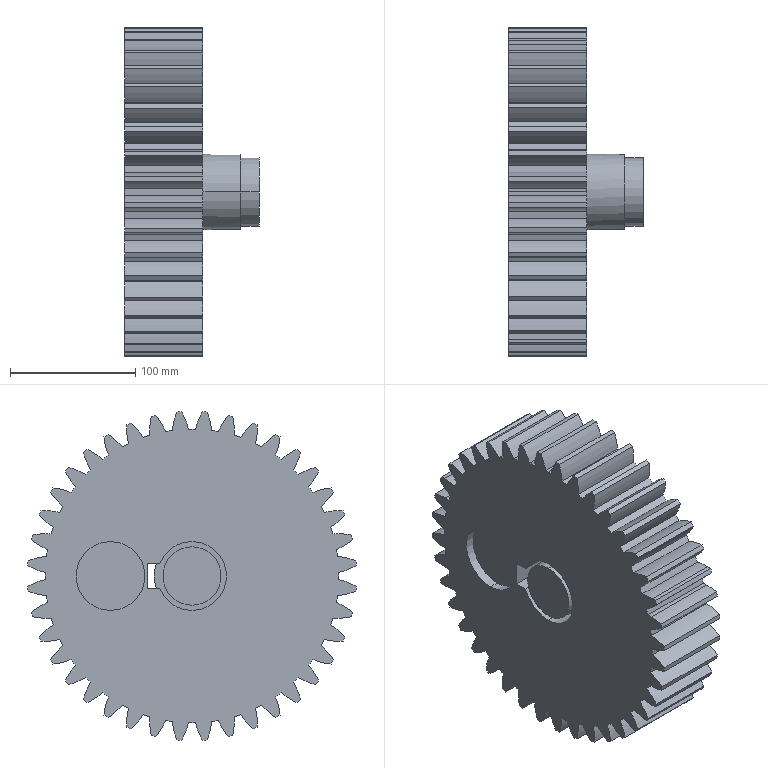Part | SolidWorks | features ICE 4, RefAxis 2, BaseBody 1, Chamfer 1, MoveFace 1, Revolution 1, Scale 1 | 2 solids | 187 faces | box 107.5 x 261.97 x 261.97 mm | volume 3068184 mm3 | cylinder 176 | plane 11 | commonest cylinder face diameters 100 x84 234.37 x41 262.5 x40 55 x7 46.517 x2 60 x2